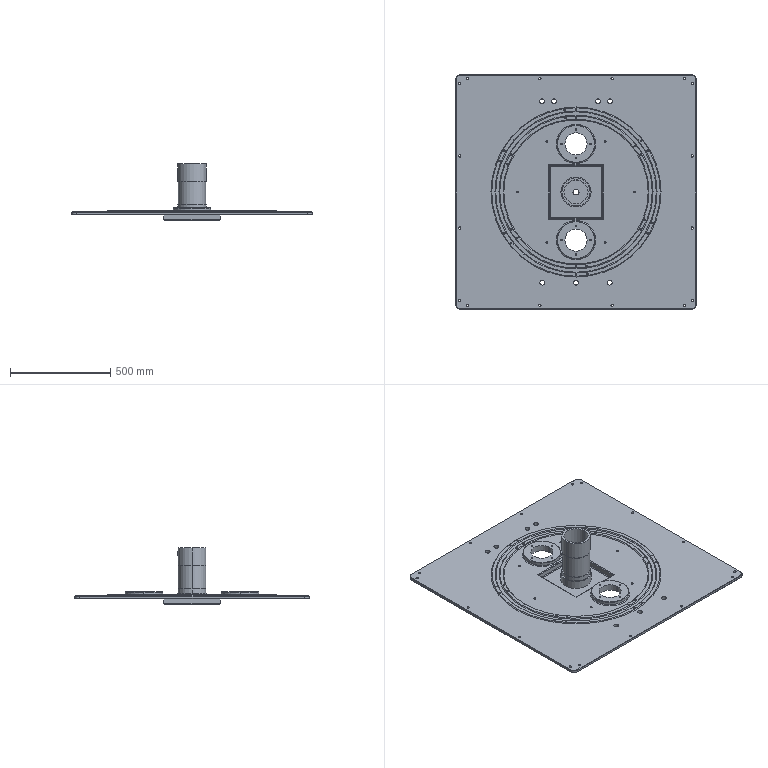Part | NX | features BREP 1 | 1 solid | 262 faces | box 1200 x 1170 x 281 mm | volume 20192903 mm3 | cylinder 177 | plane 41 | cone 28 | torus 16 | commonest cylinder face diameters 8 x76 12 x32 6.8 x16 24 x14 10 x12 48 x4